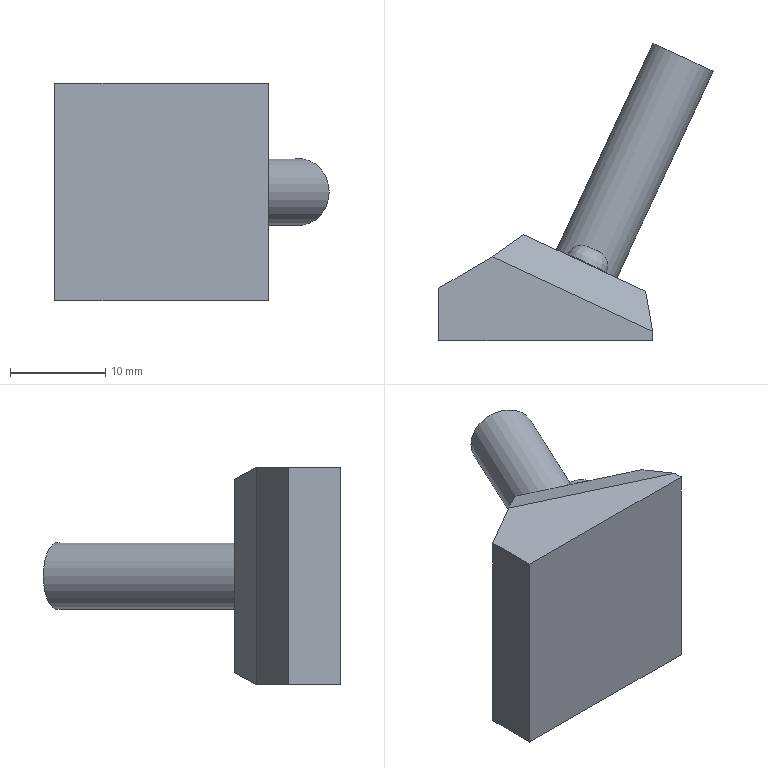Part | NX | 1 solid | 19 faces | box 28.865 x 31.283 x 22.9 mm | volume 5015 mm3 | plane 14 | cylinder 3 | spline 2 | commonest cylinder face diameters 4.5 x2 7 x1